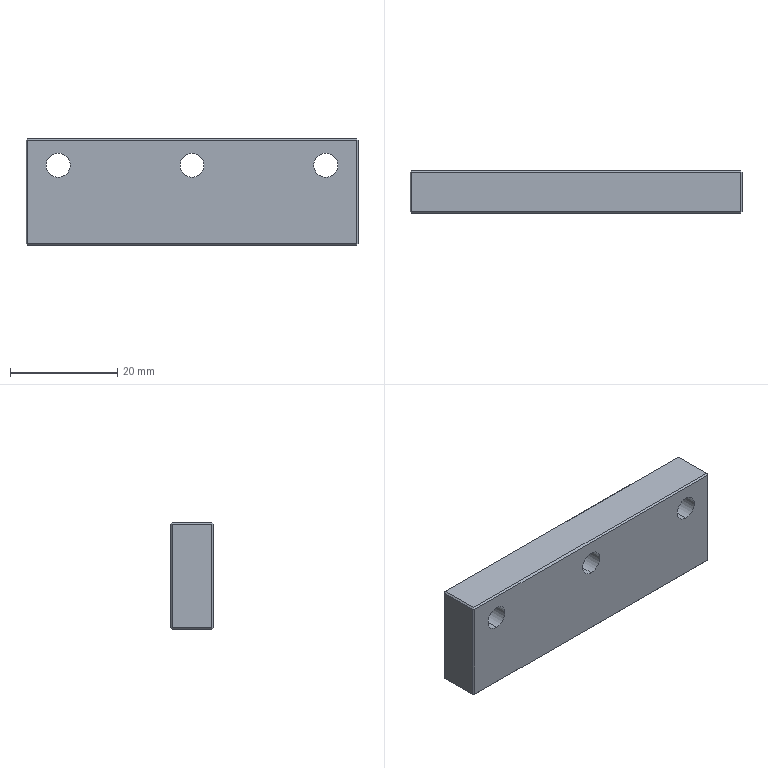Part | SolidWorks | features Chamfer 1, Extrusion 1, HoleWzd 1 | 1 solid | 41 faces | box 62 x 8 x 20 mm | volume 9069 mm3 | plane 29 | cylinder 12 | commonest cylinder face diameters 4.5 x6 8 x6
STEP:
#1=CARTESIAN_POINT('',(-25.,3.6,1.));
#2=VERTEX_POINT('',#1);
#3=CARTESIAN_POINT('',(-25.,3.6,9.));
#4=VERTEX_POINT('',#3);
#5=CARTESIAN_POINT('',(-25.,3.6,5.));
#6=DIRECTION('',(0.,1.,0.));
#7=DIRECTION('',(0.,0.,1.));
#8=AXIS2_PLACEMENT_3D('',#5,#6,#7);
#9=CIRCLE('',#8,4.);
#10=EDGE_CURVE('',#2,#4,#9,.T.);
#11=ORIENTED_EDGE('',*,*,#10,.F.);
#12=CARTESIAN_POINT('',(-25.,8.,1.));
#13=VERTEX_POINT('',#12);
#14=CARTESIAN_POINT('',(-25.,8.,1.));
#15=DIRECTION('',(0.,1.,0.));
#16=VECTOR('',#15,1000.);
#17=LINE('',#14,#16);
#18=EDGE_CURVE('',#2,#13,#17,.T.);
#19=ORIENTED_EDGE('',*,*,#18,.T.);
#20=CARTESIAN_POINT('',(-25.,8.,9.));
#21=VERTEX_POINT('',#20);
#22=CARTESIAN_POINT('',(-25.,8.,5.));
#23=DIRECTION('',(0.,1.,0.));
#24=DIRECTION('',(0.,0.,1.));
#25=AXIS2_PLACEMENT_3D('',#22,#23,#24);
#26=CIRCLE('',#25,4.);
#27=EDGE_CURVE('',#13,#21,#26,.T.);
#28=ORIENTED_EDGE('',*,*,#27,.T.);
#29=CARTESIAN_POINT('',(-25.,8.,9.));
#30=DIRECTION('',(0.,1.,0.));
#31=VECTOR('',#30,1000.);
#32=LINE('',#29,#31);
#33=EDGE_CURVE('',#4,#21,#32,.T.);
#34=ORIENTED_EDGE('',*,*,#33,.F.);
#35=EDGE_LOOP('',(#11,#19,#28,#34));
#36=FACE_OUTER_BOUND('',#35,.T.);
#37=CARTESIAN_POINT('',(-25.,8.,5.));
#38=DIRECTION('',(0.,1.,0.));
#39=DIRECTION('',(0.,0.,1.));
#40=AXIS2_PLACEMENT_3D('',#37,#38,#39);
#41=CYLINDRICAL_SURFACE('',#40,4.);
#42=ADVANCED_FACE('',(#36),#41,.F.);
#43=CARTESIAN_POINT('',(-25.,0.,2.75));
#44=VERTEX_POINT('',#43);
#45=CARTESIAN_POINT('',(-25.,0.,7.25));
#46=VERTEX_POINT('',#45);
#47=CARTESIAN_POINT('',(-25.,0.,5.));
#48=DIRECTION('',(0.,1.,0.));
#49=DIRECTION('',(0.,0.,1.));
#50=AXIS2_PLACEMENT_3D('',#47,#48,#49);
#51=CIRCLE('',#50,2.25);
#52=EDGE_CURVE('',#44,#46,#51,.T.);
#53=ORIENTED_EDGE('',*,*,#52,.F.);
#54=CARTESIAN_POINT('',(-25.,3.6,2.75));
#55=VERTEX_POINT('',#54);
#56=CARTESIAN_POINT('',(-25.,8.,2.75));
#57=DIRECTION('',(0.,1.,0.));
#58=VECTOR('',#57,1000.);
#59=LINE('',#56,#58);
#60=EDGE_CURVE('',#44,#55,#59,.T.);
#61=ORIENTED_EDGE('',*,*,#60,.T.);
#62=CARTESIAN_POINT('',(-25.,3.6,7.25));
#63=VERTEX_POINT('',#62);
#64=CARTESIAN_POINT('',(-25.,3.6,5.));
#65=DIRECTION('',(0.,1.,0.));
#66=DIRECTION('',(0.,0.,1.));
#67=AXIS2_PLACEMENT_3D('',#64,#65,#66);
#68=CIRCLE('',#67,2.25);
#69=EDGE_CURVE('',#55,#63,#68,.T.);
#70=ORIENTED_EDGE('',*,*,#69,.T.);
#71=CARTESIAN_POINT('',(-25.,8.,7.25));
#72=DIRECTION('',(0.,1.,0.));
#73=VECTOR('',#72,1000.);
#74=LINE('',#71,#73);
#75=EDGE_CURVE('',#46,#63,#74,.T.);
#76=ORIENTED_EDGE('',*,*,#75,.F.);
#77=EDGE_LOOP('',(#53,#61,#70,#76));
#78=FACE_OUTER_BOUND('',#77,.T.);
#79=CARTESIAN_POINT('',(-25.,8.,5.));
#80=DIRECTION('',(0.,1.,0.));
#81=DIRECTION('',(0.,0.,1.));
#82=AXIS2_PLACEMENT_3D('',#79,#80,#81);
#83=CYLINDRICAL_SURFACE('',#82,2.25);
#84=ADVANCED_FACE('',(#78),#83,.F.);
#85=CARTESIAN_POINT('',(0.,3.6,1.));
#86=VERTEX_POINT('',#85);
#87=CARTESIAN_POINT('',(0.,3.6,9.));
#88=VERTEX_POINT('',#87);
#89=CARTESIAN_POINT('',(0.,3.6,5.));
#90=DIRECTION('',(0.,1.,0.));
#91=DIRECTION('',(0.,0.,1.));
#92=AXIS2_PLACEMENT_3D('',#89,#90,#91);
#93=CIRCLE('',#92,4.);
#94=EDGE_CURVE('',#86,#88,#93,.T.);
#95=ORIENTED_EDGE('',*,*,#94,.F.);
#96=CARTESIAN_POINT('',(0.,8.,1.));
#97=VERTEX_POINT('',#96);
#98=CARTESIAN_POINT('',(0.,8.,1.));
#99=DIRECTION('',(0.,1.,0.));
#100=VECTOR('',#99,1000.);
#101=LINE('',#98,#100);
#102=EDGE_CURVE('',#86,#97,#101,.T.);
#103=ORIENTED_EDGE('',*,*,#102,.T.);
#104=CARTESIAN_POINT('',(0.,8.,9.));
#105=VERTEX_POINT('',#104);
#106=CARTESIAN_POINT('',(0.,8.,5.));
#107=DIRECTION('',(0.,1.,0.));
#108=DIRECTION('',(0.,0.,1.));
#109=AXIS2_PLACEMENT_3D('',#106,#107,#108);
#110=CIRCLE('',#109,4.);
#111=EDGE_CURVE('',#97,#105,#110,.T.);
#112=ORIENTED_EDGE('',*,*,#111,.T.);
#113=CARTESIAN_POINT('',(0.,8.,9.));
#114=DIRECTION('',(0.,1.,0.));
#115=VECTOR('',#114,1000.);
#116=LINE('',#113,#115);
#117=EDGE_CURVE('',#88,#105,#116,.T.);
#118=ORIENTED_EDGE('',*,*,#117,.F.);
#119=EDGE_LOOP('',(#95,#103,#112,#118));
#120=FACE_OUTER_BOUND('',#119,.T.);
#121=CARTESIAN_POINT('',(0.,8.,5.));
#122=DIRECTION('',(0.,1.,0.));
#123=DIRECTION('',(0.,0.,1.));
#124=AXIS2_PLACEMENT_3D('',#121,#122,#123);
#125=CYLINDRICAL_SURFACE('',#124,4.);
#126=ADVANCED_FACE('',(#120),#125,.F.);
#127=CARTESIAN_POINT('',(0.,0.,2.75));
#128=VERTEX_POINT('',#127);
#129=CARTESIAN_POINT('',(0.,0.,7.25));
#130=VERTEX_POINT('',#129);
#131=CARTESIAN_POINT('',(0.,0.,5.));
#132=DIRECTION('',(0.,1.,0.));
#133=DIRECTION('',(0.,0.,1.));
#134=AXIS2_PLACEMENT_3D('',#131,#132,#133);
#135=CIRCLE('',#134,2.25);
#136=EDGE_CURVE('',#128,#130,#135,.T.);
#137=ORIENTED_EDGE('',*,*,#136,.F.);
#138=CARTESIAN_POINT('',(0.,3.6,2.75));
#139=VERTEX_POINT('',#138);
#140=CARTESIAN_POINT('',(0.,8.,2.75));
#141=DIRECTION('',(0.,1.,0.));
#142=VECTOR('',#141,1000.);
#143=LINE('',#140,#142);
#144=EDGE_CURVE('',#128,#139,#143,.T.);
#145=ORIENTED_EDGE('',*,*,#144,.T.);
#146=CARTESIAN_POINT('',(0.,3.6,7.25));
#147=VERTEX_POINT('',#146);
#148=CARTESIAN_POINT('',(0.,3.6,5.));
#149=DIRECTION('',(0.,1.,0.));
#150=DIRECTION('',(0.,0.,1.));
#151=AXIS2_PLACEMENT_3D('',#148,#149,#150);
#152=CIRCLE('',#151,2.25);
#153=EDGE_CURVE('',#139,#147,#152,.T.);
#154=ORIENTED_EDGE('',*,*,#153,.T.);
#155=CARTESIAN_POINT('',(0.,8.,7.25));
#156=DIRECTION('',(0.,1.,0.));
#157=VECTOR('',#156,1000.);
#158=LINE('',#155,#157);
#159=EDGE_CURVE('',#130,#147,#158,.T.);
#160=ORIENTED_EDGE('',*,*,#159,.F.);
#161=EDGE_LOOP('',(#137,#145,#154,#160));
#162=FACE_OUTER_BOUND('',#161,.T.);
#163=CARTESIAN_POINT('',(0.,8.,5.));
#164=DIRECTION('',(0.,1.,0.));
#165=DIRECTION('',(0.,0.,1.));
#166=AXIS2_PLACEMENT_3D('',#163,#164,#165);
#167=CYLINDRICAL_SURFACE('',#166,2.25);
#168=ADVANCED_FACE('',(#162),#167,.F.);
#169=CARTESIAN_POINT('',(25.,3.6,1.));
#170=VERTEX_POINT('',#169);
#171=CARTESIAN_POINT('',(25.,3.6,9.));
#172=VERTEX_POINT('',#171);
#173=CARTESIAN_POINT('',(25.,3.6,5.));
#174=DIRECTION('',(0.,1.,0.));
#175=DIRECTION('',(0.,0.,1.));
#176=AXIS2_PLACEMENT_3D('',#173,#174,#175);
#177=CIRCLE('',#176,4.);
#178=EDGE_CURVE('',#170,#172,#177,.T.);
#179=ORIENTED_EDGE('',*,*,#178,.F.);
#180=CARTESIAN_POINT('',(25.,8.,1.));
#181=VERTEX_POINT('',#180);
#182=CARTESIAN_POINT('',(25.,8.,1.));
#183=DIRECTION('',(0.,1.,0.));
#184=VECTOR('',#183,1000.);
#185=LINE('',#182,#184);
#186=EDGE_CURVE('',#170,#181,#185,.T.);
#187=ORIENTED_EDGE('',*,*,#186,.T.);
#188=CARTESIAN_POINT('',(25.,8.,9.));
#189=VERTEX_POINT('',#188);
#190=CARTESIAN_POINT('',(25.,8.,5.));
#191=DIRECTION('',(0.,1.,0.));
#192=DIRECTION('',(0.,0.,1.));
#193=AXIS2_PLACEMENT_3D('',#190,#191,#192);
#194=CIRCLE('',#193,4.);
#195=EDGE_CURVE('',#181,#189,#194,.T.);
#196=ORIENTED_EDGE('',*,*,#195,.T.);
#197=CARTESIAN_POINT('',(25.,8.,9.));
#198=DIRECTION('',(0.,1.,0.));
#199=VECTOR('',#198,1000.);
#200=LINE('',#197,#199);
#201=EDGE_CURVE('',#172,#189,#200,.T.);
#202=ORIENTED_EDGE('',*,*,#201,.F.);
#203=EDGE_LOOP('',(#179,#187,#196,#202));
#204=FACE_OUTER_BOUND('',#203,.T.);
#205=CARTESIAN_POINT('',(25.,8.,5.));
#206=DIRECTION('',(0.,1.,0.));
#207=DIRECTION('',(0.,0.,1.));
#208=AXIS2_PLACEMENT_3D('',#205,#206,#207);
#209=CYLINDRICAL_SURFACE('',#208,4.);
#210=ADVANCED_FACE('',(#204),#209,.F.);
#211=CARTESIAN_POINT('',(25.,0.,2.75));
#212=VERTEX_POINT('',#211);
#213=CARTESIAN_POINT('',(25.,0.,7.25));
#214=VERTEX_POINT('',#213);
#215=CARTESIAN_POINT('',(25.,0.,5.));
#216=DIRECTION('',(0.,1.,0.));
#217=DIRECTION('',(0.,0.,1.));
#218=AXIS2_PLACEMENT_3D('',#215,#216,#217);
#219=CIRCLE('',#218,2.25);
#220=EDGE_CURVE('',#212,#214,#219,.T.);
#221=ORIENTED_EDGE('',*,*,#220,.F.);
#222=CARTESIAN_POINT('',(25.,3.6,2.75));
#223=VERTEX_POINT('',#222);
#224=CARTESIAN_POINT('',(25.,8.,2.75));
#225=DIRECTION('',(0.,1.,0.));
#226=VECTOR('',#225,1000.);
#227=LINE('',#224,#226);
#228=EDGE_CURVE('',#212,#223,#227,.T.);
#229=ORIENTED_EDGE('',*,*,#228,.T.);
#230=CARTESIAN_POINT('',(25.,3.6,7.25));
#231=VERTEX_POINT('',#230);
#232=CARTESIAN_POINT('',(25.,3.6,5.));
#233=DIRECTION('',(0.,1.,0.));
#234=DIRECTION('',(0.,0.,1.));
#235=AXIS2_PLACEMENT_3D('',#232,#233,#234);
#236=CIRCLE('',#235,2.25);
#237=EDGE_CURVE('',#223,#231,#236,.T.);
#238=ORIENTED_EDGE('',*,*,#237,.T.);
#239=CARTESIAN_POINT('',(25.,8.,7.25));
#240=DIRECTION('',(0.,1.,0.));
#241=VECTOR('',#240,1000.);
#242=LINE('',#239,#241);
#243=EDGE_CURVE('',#214,#231,#242,.T.);
#244=ORIENTED_EDGE('',*,*,#243,.F.);
#245=EDGE_LOOP('',(#221,#229,#238,#244));
#246=FACE_OUTER_BOUND('',#245,.T.);
#247=CARTESIAN_POINT('',(25.,8.,5.));
#248=DIRECTION('',(0.,1.,0.));
#249=DIRECTION('',(0.,0.,1.));
#250=AXIS2_PLACEMENT_3D('',#247,#248,#249);
#251=CYLINDRICAL_SURFACE('',#250,2.25);
#252=ADVANCED_FACE('',(#246),#251,.F.);
#253=CARTESIAN_POINT('',(31.,0.3,-9.7));
#254=VERTEX_POINT('',#253);
#255=CARTESIAN_POINT('',(31.,7.7,-9.7));
#256=VERTEX_POINT('',#255);
#257=CARTESIAN_POINT('',(31.,8.,-9.7));
#258=DIRECTION('',(0.,1.,0.));
#259=VECTOR('',#258,1000.);
#260=LINE('',#257,#259);
#261=EDGE_CURVE('',#254,#256,#260,.T.);
#262=ORIENTED_EDGE('',*,*,#261,.T.);
#263=CARTESIAN_POINT('',(31.,7.7,9.7));
#264=VERTEX_POINT('',#263);
#265=CARTESIAN_POINT('',(31.,7.7,10.));
#266=DIRECTION('',(0.,0.,1.));
#267=VECTOR('',#266,1000.);
#268=LINE('',#265,#267);
#269=EDGE_CURVE('',#256,#264,#268,.T.);
#270=ORIENTED_EDGE('',*,*,#269,.T.);
#271=CARTESIAN_POINT('',(31.,0.3,9.7));
#272=VERTEX_POINT('',#271);
#273=CARTESIAN_POINT('',(31.,8.,9.7));
#274=DIRECTION('',(0.,-1.,0.));
#275=VECTOR('',#274,1000.);
#276=LINE('',#273,#275);
#277=EDGE_CURVE('',#264,#272,#276,.T.);
#278=ORIENTED_EDGE('',*,*,#277,.T.);
#279=CARTESIAN_POINT('',(31.,0.3,-10.));
#280=DIRECTION('',(0.,0.,-1.));
#281=VECTOR('',#280,1000.);
#282=LINE('',#279,#281);
#283=EDGE_CURVE('',#272,#254,#282,.T.);
#284=ORIENTED_EDGE('',*,*,#283,.T.);
#285=EDGE_LOOP('',(#262,#270,#278,#284));
#286=FACE_OUTER_BOUND('',#285,.T.);
#287=CARTESIAN_POINT('',(31.,8.,-10.));
#288=DIRECTION('',(-1.,0.,0.));
#289=DIRECTION('',(0.,0.,1.));
#290=AXIS2_PLACEMENT_3D('',#287,#288,#289);
#291=PLANE('',#290);
#292=ADVANCED_FACE('',(#286),#291,.F.);
#293=CARTESIAN_POINT('',(-30.7,0.3,-10.));
#294=VERTEX_POINT('',#293);
#295=CARTESIAN_POINT('',(-30.7,7.7,-10.));
#296=VERTEX_POINT('',#295);
#297=CARTESIAN_POINT('',(-30.7,8.,-10.));
#298=DIRECTION('',(0.,1.,0.));
#299=VECTOR('',#298,1000.);
#300=LINE('',#297,#299);
#301=EDGE_CURVE('',#294,#296,#300,.T.);
#302=ORIENTED_EDGE('',*,*,#301,.T.);
#303=CARTESIAN_POINT('',(30.7,7.7,-10.));
#304=VERTEX_POINT('',#303);
#305=CARTESIAN_POINT('',(31.,7.7,-10.));
#306=DIRECTION('',(1.,0.,0.));
#307=VECTOR('',#306,1000.);
#308=LINE('',#305,#307);
#309=EDGE_CURVE('',#296,#304,#308,.T.);
#310=ORIENTED_EDGE('',*,*,#309,.T.);
#311=CARTESIAN_POINT('',(30.7,0.3,-10.));
#312=VERTEX_POINT('',#311);
#313=CARTESIAN_POINT('',(30.7,8.,-10.));
#314=DIRECTION('',(0.,-1.,0.));
#315=VECTOR('',#314,1000.);
#316=LINE('',#313,#315);
#317=EDGE_CURVE('',#304,#312,#316,.T.);
#318=ORIENTED_EDGE('',*,*,#317,.T.);
#319=CARTESIAN_POINT('',(-31.,0.3,-10.));
#320=DIRECTION('',(-1.,0.,0.));
#321=VECTOR('',#320,1000.);
#322=LINE('',#319,#321);
#323=EDGE_CURVE('',#312,#294,#322,.T.);
#324=ORIENTED_EDGE('',*,*,#323,.T.);
#325=EDGE_LOOP('',(#302,#310,#318,#324));
#326=FACE_OUTER_BOUND('',#325,.T.);
#327=CARTESIAN_POINT('',(-31.,8.,-10.));
#328=DIRECTION('',(0.,0.,1.));
#329=DIRECTION('',(1.,0.,0.));
#330=AXIS2_PLACEMENT_3D('',#327,#328,#329);
#331=PLANE('',#330);
#332=ADVANCED_FACE('',(#326),#331,.F.);
#333=CARTESIAN_POINT('',(-31.,7.7,9.7));
#334=VERTEX_POINT('',#333);
#335=CARTESIAN_POINT('',(-31.,7.7,-9.7));
#336=VERTEX_POINT('',#335);
#337=CARTESIAN_POINT('',(-31.,7.7,-10.));
#338=DIRECTION('',(0.,0.,-1.));
#339=VECTOR('',#338,1000.);
#340=LINE('',#337,#339);
#341=EDGE_CURVE('',#334,#336,#340,.T.);
#342=ORIENTED_EDGE('',*,*,#341,.T.);
#343=CARTESIAN_POINT('',(-31.,0.3,-9.7));
#344=VERTEX_POINT('',#343);
#345=CARTESIAN_POINT('',(-31.,8.,-9.7));
#346=DIRECTION('',(0.,-1.,0.));
#347=VECTOR('',#346,1000.);
#348=LINE('',#345,#347);
#349=EDGE_CURVE('',#336,#344,#348,.T.);
#350=ORIENTED_EDGE('',*,*,#349,.T.);
#351=CARTESIAN_POINT('',(-31.,0.3,9.7));
#352=VERTEX_POINT('',#351);
#353=CARTESIAN_POINT('',(-31.,0.3,-10.));
#354=DIRECTION('',(0.,0.,1.));
#355=VECTOR('',#354,1000.);
#356=LINE('',#353,#355);
#357=EDGE_CURVE('',#344,#352,#356,.T.);
#358=ORIENTED_EDGE('',*,*,#357,.T.);
#359=CARTESIAN_POINT('',(-31.,8.,9.7));
#360=DIRECTION('',(0.,1.,0.));
#361=VECTOR('',#360,1000.);
#362=LINE('',#359,#361);
#363=EDGE_CURVE('',#352,#334,#362,.T.);
#364=ORIENTED_EDGE('',*,*,#363,.T.);
#365=EDGE_LOOP('',(#342,#350,#358,#364));
#366=FACE_OUTER_BOUND('',#365,.T.);
#367=CARTESIAN_POINT('',(-31.,8.,-10.));
#368=DIRECTION('',(1.,0.,0.));
#369=DIRECTION('',(0.,0.,-1.));
#370=AXIS2_PLACEMENT_3D('',#367,#368,#369);
#371=PLANE('',#370);
#372=ADVANCED_FACE('',(#366),#371,.F.);
#373=CARTESIAN_POINT('',(30.7,7.7,10.));
#374=VERTEX_POINT('',#373);
#375=CARTESIAN_POINT('',(-30.7,7.7,10.));
#376=VERTEX_POINT('',#375);
#377=CARTESIAN_POINT('',(-31.,7.7,10.));
#378=DIRECTION('',(-1.,0.,0.));
#379=VECTOR('',#378,1000.);
#380=LINE('',#377,#379);
#381=EDGE_CURVE('',#374,#376,#380,.T.);
#382=ORIENTED_EDGE('',*,*,#381,.T.);
#383=CARTESIAN_POINT('',(-30.7,0.3,10.));
#384=VERTEX_POINT('',#383);
#385=CARTESIAN_POINT('',(-30.7,8.,10.));
#386=DIRECTION('',(0.,-1.,0.));
#387=VECTOR('',#386,1000.);
#388=LINE('',#385,#387);
#389=EDGE_CURVE('',#376,#384,#388,.T.);
#390=ORIENTED_EDGE('',*,*,#389,.T.);
#391=CARTESIAN_POINT('',(30.7,0.3,10.));
#392=VERTEX_POINT('',#391);
#393=CARTESIAN_POINT('',(-31.,0.3,10.));
#394=DIRECTION('',(1.,0.,0.));
#395=VECTOR('',#394,1000.);
#396=LINE('',#393,#395);
#397=EDGE_CURVE('',#384,#392,#396,.T.);
#398=ORIENTED_EDGE('',*,*,#397,.T.);
#399=CARTESIAN_POINT('',(30.7,8.,10.));
#400=DIRECTION('',(0.,1.,0.));
#401=VECTOR('',#400,1000.);
#402=LINE('',#399,#401);
#403=EDGE_CURVE('',#392,#374,#402,.T.);
#404=ORIENTED_EDGE('',*,*,#403,.T.);
#405=EDGE_LOOP('',(#382,#390,#398,#404));
#406=FACE_OUTER_BOUND('',#405,.T.);
#407=CARTESIAN_POINT('',(-31.,8.,10.));
#408=DIRECTION('',(0.,0.,-1.));
#409=DIRECTION('',(-1.,0.,0.));
#410=AXIS2_PLACEMENT_3D('',#407,#408,#409);
#411=PLANE('',#410);
#412=ADVANCED_FACE('',(#406),#411,.F.);
#413=CARTESIAN_POINT('',(30.7,8.,-9.7));
#414=VERTEX_POINT('',#413);
#415=CARTESIAN_POINT('',(-30.7,8.,-9.7));
#416=VERTEX_POINT('',#415);
#417=CARTESIAN_POINT('',(-31.,8.,-9.7));
#418=DIRECTION('',(-1.,0.,0.));
#419=VECTOR('',#418,1000.);
#420=LINE('',#417,#419);
#421=EDGE_CURVE('',#414,#416,#420,.T.);
#422=ORIENTED_EDGE('',*,*,#421,.T.);
#423=CARTESIAN_POINT('',(-30.7,8.,9.7));
#424=VERTEX_POINT('',#423);
#425=CARTESIAN_POINT('',(-30.7,8.,10.));
#426=DIRECTION('',(0.,0.,1.));
#427=VECTOR('',#426,1000.);
#428=LINE('',#425,#427);
#429=EDGE_CURVE('',#416,#424,#428,.T.);
#430=ORIENTED_EDGE('',*,*,#429,.T.);
#431=CARTESIAN_POINT('',(30.7,8.,9.7));
#432=VERTEX_POINT('',#431);
#433=CARTESIAN_POINT('',(31.,8.,9.7));
#434=DIRECTION('',(1.,0.,0.));
#435=VECTOR('',#434,1000.);
#436=LINE('',#433,#435);
#437=EDGE_CURVE('',#424,#432,#436,.T.);
#438=ORIENTED_EDGE('',*,*,#437,.T.);
#439=CARTESIAN_POINT('',(30.7,8.,-10.));
#440=DIRECTION('',(0.,0.,-1.));
#441=VECTOR('',#440,1000.);
#442=LINE('',#439,#441);
#443=EDGE_CURVE('',#432,#414,#442,.T.);
#444=ORIENTED_EDGE('',*,*,#443,.T.);
#445=EDGE_LOOP('',(#422,#430,#438,#444));
#446=FACE_OUTER_BOUND('',#445,.T.);
#447=CARTESIAN_POINT('',(-25.,8.,5.));
#448=DIRECTION('',(0.,1.,0.));
#449=DIRECTION('',(0.,0.,1.));
#450=AXIS2_PLACEMENT_3D('',#447,#448,#449);
#451=CIRCLE('',#450,4.);
#452=EDGE_CURVE('',#21,#13,#451,.T.);
#453=ORIENTED_EDGE('',*,*,#452,.F.);
#454=ORIENTED_EDGE('',*,*,#27,.F.);
#455=EDGE_LOOP('',(#453,#454));
#456=FACE_BOUND('',#455,.T.);
#457=CARTESIAN_POINT('',(0.,8.,5.));
#458=DIRECTION('',(0.,1.,0.));
#459=DIRECTION('',(0.,0.,1.));
#460=AXIS2_PLACEMENT_3D('',#457,#458,#459);
#461=CIRCLE('',#460,4.);
#462=EDGE_CURVE('',#105,#97,#461,.T.);
#463=ORIENTED_EDGE('',*,*,#462,.F.);
#464=ORIENTED_EDGE('',*,*,#111,.F.);
#465=EDGE_LOOP('',(#463,#464));
#466=FACE_BOUND('',#465,.T.);
#467=CARTESIAN_POINT('',(25.,8.,5.));
#468=DIRECTION('',(0.,1.,0.));
#469=DIRECTION('',(0.,0.,1.));
#470=AXIS2_PLACEMENT_3D('',#467,#468,#469);
#471=CIRCLE('',#470,4.);
#472=EDGE_CURVE('',#189,#181,#471,.T.);
#473=ORIENTED_EDGE('',*,*,#472,.F.);
#474=ORIENTED_EDGE('',*,*,#195,.F.);
#475=EDGE_LOOP('',(#473,#474));
#476=FACE_BOUND('',#475,.T.);
#477=CARTESIAN_POINT('',(0.,8.,0.));
#478=DIRECTION('',(0.,1.,0.));
#479=DIRECTION('',(0.,0.,1.));
#480=AXIS2_PLACEMENT_3D('',#477,#478,#479);
#481=PLANE('',#480);
#482=ADVANCED_FACE('',(#446,#456,#466,#476),#481,.T.);
#483=CARTESIAN_POINT('',(30.7,0.,9.7));
#484=VERTEX_POINT('',#483);
#485=CARTESIAN_POINT('',(-30.7,0.,9.7));
#486=VERTEX_POINT('',#485);
#487=CARTESIAN_POINT('',(0.,0.,9.7));
#488=DIRECTION('',(-1.,0.,0.));
#489=VECTOR('',#488,1000.);
#490=LINE('',#487,#489);
#491=EDGE_CURVE('',#484,#486,#490,.T.);
#492=ORIENTED_EDGE('',*,*,#491,.T.);
#493=CARTESIAN_POINT('',(-30.7,0.,-9.7));
#494=VERTEX_POINT('',#493);
#495=CARTESIAN_POINT('',(-30.7,0.,0.));
#496=DIRECTION('',(0.,0.,-1.));
#497=VECTOR('',#496,1000.);
#498=LINE('',#495,#497);
#499=EDGE_CURVE('',#486,#494,#498,.T.);
#500=ORIENTED_EDGE('',*,*,#499,.T.);
#501=CARTESIAN_POINT('',(30.7,0.,-9.7));
#502=VERTEX_POINT('',#501);
#503=CARTESIAN_POINT('',(0.,0.,-9.7));
#504=DIRECTION('',(1.,0.,0.));
#505=VECTOR('',#504,1000.);
#506=LINE('',#503,#505);
#507=EDGE_CURVE('',#494,#502,#506,.T.);
#508=ORIENTED_EDGE('',*,*,#507,.T.);
#509=CARTESIAN_POINT('',(30.7,0.,0.));
#510=DIRECTION('',(0.,0.,1.));
#511=VECTOR('',#510,1000.);
#512=LINE('',#509,#511);
#513=EDGE_CURVE('',#502,#484,#512,.T.);
#514=ORIENTED_EDGE('',*,*,#513,.T.);
#515=EDGE_LOOP('',(#492,#500,#508,#514));
#516=FACE_OUTER_BOUND('',#515,.T.);
#517=CARTESIAN_POINT('',(-25.,0.,5.));
#518=DIRECTION('',(0.,1.,0.));
#519=DIRECTION('',(0.,0.,1.));
#520=AXIS2_PLACEMENT_3D('',#517,#518,#519);
#521=CIRCLE('',#520,2.25);
#522=EDGE_CURVE('',#46,#44,#521,.T.);
#523=ORIENTED_EDGE('',*,*,#522,.T.);
#524=ORIENTED_EDGE('',*,*,#52,.T.);
#525=EDGE_LOOP('',(#523,#524));
#526=FACE_BOUND('',#525,.T.);
#527=CARTESIAN_POINT('',(0.,0.,5.));
#528=DIRECTION('',(0.,1.,0.));
#529=DIRECTION('',(0.,0.,1.));
#530=AXIS2_PLACEMENT_3D('',#527,#528,#529);
#531=CIRCLE('',#530,2.25);
#532=EDGE_CURVE('',#130,#128,#531,.T.);
#533=ORIENTED_EDGE('',*,*,#532,.T.);
#534=ORIENTED_EDGE('',*,*,#136,.T.);
#535=EDGE_LOOP('',(#533,#534));
#536=FACE_BOUND('',#535,.T.);
#537=CARTESIAN_POINT('',(25.,0.,5.));
#538=DIRECTION('',(0.,1.,0.));
#539=DIRECTION('',(0.,0.,1.));
#540=AXIS2_PLACEMENT_3D('',#537,#538,#539);
#541=CIRCLE('',#540,2.25);
#542=EDGE_CURVE('',#214,#212,#541,.T.);
#543=ORIENTED_EDGE('',*,*,#542,.T.);
#544=ORIENTED_EDGE('',*,*,#220,.T.);
#545=EDGE_LOOP('',(#543,#544));
#546=FACE_BOUND('',#545,.T.);
#547=CARTESIAN_POINT('',(0.,0.,0.));
#548=DIRECTION('',(0.,1.,0.));
#549=DIRECTION('',(0.,0.,1.));
#550=AXIS2_PLACEMENT_3D('',#547,#548,#549);
#551=PLANE('',#550);
#552=ADVANCED_FACE('',(#516,#526,#536,#546),#551,.F.);
#553=ORIENTED_EDGE('',*,*,#228,.F.);
#554=ORIENTED_EDGE('',*,*,#542,.F.);
#555=ORIENTED_EDGE('',*,*,#243,.T.);
#556=CARTESIAN_POINT('',(25.,3.6,5.));
#557=DIRECTION('',(0.,1.,0.));
#558=DIRECTION('',(0.,0.,1.));
#559=AXIS2_PLACEMENT_3D('',#556,#557,#558);
#560=CIRCLE('',#559,2.25);
#561=EDGE_CURVE('',#231,#223,#560,.T.);
#562=ORIENTED_EDGE('',*,*,#561,.T.);
#563=EDGE_LOOP('',(#553,#554,#555,#562));
#564=FACE_OUTER_BOUND('',#563,.T.);
#565=CARTESIAN_POINT('',(25.,8.,5.));
#566=DIRECTION('',(0.,1.,0.));
#567=DIRECTION('',(0.,0.,1.));
#568=AXIS2_PLACEMENT_3D('',#565,#566,#567);
#569=CYLINDRICAL_SURFACE('',#568,2.25);
#570=ADVANCED_FACE('',(#564),#569,.F.);
#571=ORIENTED_EDGE('',*,*,#561,.F.);
#572=ORIENTED_EDGE('',*,*,#237,.F.);
#573=EDGE_LOOP('',(#571,#572));
#574=FACE_BOUND('',#573,.T.);
#575=CARTESIAN_POINT('',(25.,3.6,5.));
#576=DIRECTION('',(0.,1.,0.));
#577=DIRECTION('',(0.,0.,1.));
#578=AXIS2_PLACEMENT_3D('',#575,#576,#577);
#579=CIRCLE('',#578,4.);
#580=EDGE_CURVE('',#172,#170,#579,.T.);
#581=ORIENTED_EDGE('',*,*,#580,.T.);
#582=ORIENTED_EDGE('',*,*,#178,.T.);
#583=EDGE_LOOP('',(#581,#582));
#584=FACE_OUTER_BOUND('',#583,.T.);
#585=CARTESIAN_POINT('',(27.25,3.6,5.));
#586=DIRECTION('',(0.,-1.,0.));
#587=DIRECTION('',(0.,0.,-1.));
#588=AXIS2_PLACEMENT_3D('',#585,#586,#587);
#589=PLANE('',#588);
#590=ADVANCED_FACE('',(#574,#584),#589,.F.);
#591=ORIENTED_EDGE('',*,*,#186,.F.);
#592=ORIENTED_EDGE('',*,*,#580,.F.);
#593=ORIENTED_EDGE('',*,*,#201,.T.);
#594=ORIENTED_EDGE('',*,*,#472,.T.);
#595=EDGE_LOOP('',(#591,#592,#593,#594));
#596=FACE_OUTER_BOUND('',#595,.T.);
#597=CARTESIAN_POINT('',(25.,8.,5.));
#598=DIRECTION('',(0.,1.,0.));
#599=DIRECTION('',(0.,0.,1.));
#600=AXIS2_PLACEMENT_3D('',#597,#598,#599);
#601=CYLINDRICAL_SURFACE('',#600,4.);
#602=ADVANCED_FACE('',(#596),#601,.F.);
#603=ORIENTED_EDGE('',*,*,#144,.F.);
#604=ORIENTED_EDGE('',*,*,#532,.F.);
#605=ORIENTED_EDGE('',*,*,#159,.T.);
#606=CARTESIAN_POINT('',(0.,3.6,5.));
#607=DIRECTION('',(0.,1.,0.));
#608=DIRECTION('',(0.,0.,1.));
#609=AXIS2_PLACEMENT_3D('',#606,#607,#608);
#610=CIRCLE('',#609,2.25);
#611=EDGE_CURVE('',#147,#139,#610,.T.);
#612=ORIENTED_EDGE('',*,*,#611,.T.);
#613=EDGE_LOOP('',(#603,#604,#605,#612));
#614=FACE_OUTER_BOUND('',#613,.T.);
#615=CARTESIAN_POINT('',(0.,8.,5.));
#616=DIRECTION('',(0.,1.,0.));
#617=DIRECTION('',(0.,0.,1.));
#618=AXIS2_PLACEMENT_3D('',#615,#616,#617);
#619=CYLINDRICAL_SURFACE('',#618,2.25);
#620=ADVANCED_FACE('',(#614),#619,.F.);
#621=ORIENTED_EDGE('',*,*,#611,.F.);
#622=ORIENTED_EDGE('',*,*,#153,.F.);
#623=EDGE_LOOP('',(#621,#622));
#624=FACE_BOUND('',#623,.T.);
#625=CARTESIAN_POINT('',(0.,3.6,5.));
#626=DIRECTION('',(0.,1.,0.));
#627=DIRECTION('',(0.,0.,1.));
#628=AXIS2_PLACEMENT_3D('',#625,#626,#627);
#629=CIRCLE('',#628,4.);
#630=EDGE_CURVE('',#88,#86,#629,.T.);
#631=ORIENTED_EDGE('',*,*,#630,.T.);
#632=ORIENTED_EDGE('',*,*,#94,.T.);
#633=EDGE_LOOP('',(#631,#632));
#634=FACE_OUTER_BOUND('',#633,.T.);
#635=CARTESIAN_POINT('',(2.25,3.6,5.));
#636=DIRECTION('',(0.,-1.,0.));
#637=DIRECTION('',(0.,0.,-1.));
#638=AXIS2_PLACEMENT_3D('',#635,#636,#637);
#639=PLANE('',#638);
#640=ADVANCED_FACE('',(#624,#634),#639,.F.);
#641=ORIENTED_EDGE('',*,*,#102,.F.);
#642=ORIENTED_EDGE('',*,*,#630,.F.);
#643=ORIENTED_EDGE('',*,*,#117,.T.);
#644=ORIENTED_EDGE('',*,*,#462,.T.);
#645=EDGE_LOOP('',(#641,#642,#643,#644));
#646=FACE_OUTER_BOUND('',#645,.T.);
#647=CARTESIAN_POINT('',(0.,8.,5.));
#648=DIRECTION('',(0.,1.,0.));
#649=DIRECTION('',(0.,0.,1.));
#650=AXIS2_PLACEMENT_3D('',#647,#648,#649);
#651=CYLINDRICAL_SURFACE('',#650,4.);
#652=ADVANCED_FACE('',(#646),#651,.F.);
#653=ORIENTED_EDGE('',*,*,#60,.F.);
#654=ORIENTED_EDGE('',*,*,#522,.F.);
#655=ORIENTED_EDGE('',*,*,#75,.T.);
#656=CARTESIAN_POINT('',(-25.,3.6,5.));
#657=DIRECTION('',(0.,1.,0.));
#658=DIRECTION('',(0.,0.,1.));
#659=AXIS2_PLACEMENT_3D('',#656,#657,#658);
#660=CIRCLE('',#659,2.25);
#661=EDGE_CURVE('',#63,#55,#660,.T.);
#662=ORIENTED_EDGE('',*,*,#661,.T.);
#663=EDGE_LOOP('',(#653,#654,#655,#662));
#664=FACE_OUTER_BOUND('',#663,.T.);
#665=CARTESIAN_POINT('',(-25.,8.,5.));
#666=DIRECTION('',(0.,1.,0.));
#667=DIRECTION('',(0.,0.,1.));
#668=AXIS2_PLACEMENT_3D('',#665,#666,#667);
#669=CYLINDRICAL_SURFACE('',#668,2.25);
#670=ADVANCED_FACE('',(#664),#669,.F.);
#671=ORIENTED_EDGE('',*,*,#661,.F.);
#672=ORIENTED_EDGE('',*,*,#69,.F.);
#673=EDGE_LOOP('',(#671,#672));
#674=FACE_BOUND('',#673,.T.);
#675=CARTESIAN_POINT('',(-25.,3.6,5.));
#676=DIRECTION('',(0.,1.,0.));
#677=DIRECTION('',(0.,0.,1.));
#678=AXIS2_PLACEMENT_3D('',#675,#676,#677);
#679=CIRCLE('',#678,4.);
#680=EDGE_CURVE('',#4,#2,#679,.T.);
#681=ORIENTED_EDGE('',*,*,#680,.T.);
#682=ORIENTED_EDGE('',*,*,#10,.T.);
#683=EDGE_LOOP('',(#681,#682));
#684=FACE_OUTER_BOUND('',#683,.T.);
#685=CARTESIAN_POINT('',(-22.75,3.6,5.));
#686=DIRECTION('',(0.,-1.,0.));
#687=DIRECTION('',(0.,0.,-1.));
#688=AXIS2_PLACEMENT_3D('',#685,#686,#687);
#689=PLANE('',#688);
#690=ADVANCED_FACE('',(#674,#684),#689,.F.);
#691=ORIENTED_EDGE('',*,*,#18,.F.);
#692=ORIENTED_EDGE('',*,*,#680,.F.);
#693=ORIENTED_EDGE('',*,*,#33,.T.);
#694=ORIENTED_EDGE('',*,*,#452,.T.);
#695=EDGE_LOOP('',(#691,#692,#693,#694));
#696=FACE_OUTER_BOUND('',#695,.T.);
#697=CARTESIAN_POINT('',(-25.,8.,5.));
#698=DIRECTION('',(0.,1.,0.));
#699=DIRECTION('',(0.,0.,1.));
#700=AXIS2_PLACEMENT_3D('',#697,#698,#699);
#701=CYLINDRICAL_SURFACE('',#700,4.);
#702=ADVANCED_FACE('',(#696),#701,.F.);
#703=CARTESIAN_POINT('',(30.7,0.,-9.7));
#704=DIRECTION('',(-0.7071,-0.7071,0.));
#705=VECTOR('',#704,1000.);
#706=LINE('',#703,#705);
#707=EDGE_CURVE('',#254,#502,#706,.T.);
#708=ORIENTED_EDGE('',*,*,#707,.F.);
#709=ORIENTED_EDGE('',*,*,#283,.F.);
#710=CARTESIAN_POINT('',(30.7,0.,9.7));
#711=DIRECTION('',(0.7071,0.7071,0.));
#712=VECTOR('',#711,1000.);
#713=LINE('',#710,#712);
#714=EDGE_CURVE('',#484,#272,#713,.T.);
#715=ORIENTED_EDGE('',*,*,#714,.F.);
#716=ORIENTED_EDGE('',*,*,#513,.F.);
#717=EDGE_LOOP('',(#708,#709,#715,#716));
#718=FACE_OUTER_BOUND('',#717,.T.);
#719=CARTESIAN_POINT('',(31.,0.3,-10.));
#720=DIRECTION('',(-0.7071,0.7071,0.));
#721=DIRECTION('',(0.,0.,-1.));
#722=AXIS2_PLACEMENT_3D('',#719,#720,#721);
#723=PLANE('',#722);
#724=ADVANCED_FACE('',(#718),#723,.F.);
#725=CARTESIAN_POINT('',(30.85,0.3,-9.85));
#726=DIRECTION('',(-0.7071,0.,-0.7071));
#727=VECTOR('',#726,1000.);
#728=LINE('',#725,#727);
#729=EDGE_CURVE('',#254,#312,#728,.T.);
#730=ORIENTED_EDGE('',*,*,#729,.F.);
#731=ORIENTED_EDGE('',*,*,#707,.T.);
#732=CARTESIAN_POINT('',(30.7,0.,-9.7));
#733=DIRECTION('',(0.,-0.7071,0.7071));
#734=VECTOR('',#733,1000.);
#735=LINE('',#732,#734);
#736=EDGE_CURVE('',#312,#502,#735,.T.);
#737=ORIENTED_EDGE('',*,*,#736,.F.);
#738=EDGE_LOOP('',(#730,#731,#737));
#739=FACE_OUTER_BOUND('',#738,.T.);
#740=CARTESIAN_POINT('',(30.7,0.,-9.7));
#741=DIRECTION('',(0.5774,-0.5774,-0.5774));
#742=DIRECTION('',(0.7071,0.7071,0.));
#743=AXIS2_PLACEMENT_3D('',#740,#741,#742);
#744=PLANE('',#743);
#745=ADVANCED_FACE('',(#739),#744,.T.);
#746=CARTESIAN_POINT('',(30.7,0.,9.7));
#747=DIRECTION('',(0.,0.7071,0.7071));
#748=VECTOR('',#747,1000.);
#749=LINE('',#746,#748);
#750=EDGE_CURVE('',#484,#392,#749,.T.);
#751=ORIENTED_EDGE('',*,*,#750,.F.);
#752=ORIENTED_EDGE('',*,*,#714,.T.);
#753=CARTESIAN_POINT('',(30.85,0.3,9.85));
#754=DIRECTION('',(0.7071,0.,-0.7071));
#755=VECTOR('',#754,1000.);
#756=LINE('',#753,#755);
#757=EDGE_CURVE('',#392,#272,#756,.T.);
#758=ORIENTED_EDGE('',*,*,#757,.F.);
#759=EDGE_LOOP('',(#751,#752,#758));
#760=FACE_OUTER_BOUND('',#759,.T.);
#761=CARTESIAN_POINT('',(30.7,0.,9.7));
#762=DIRECTION('',(0.5774,-0.5774,0.5774));
#763=DIRECTION('',(0.7071,0.7071,0.));
#764=AXIS2_PLACEMENT_3D('',#761,#762,#763);
#765=PLANE('',#764);
#766=ADVANCED_FACE('',(#760),#765,.T.);
#767=ORIENTED_EDGE('',*,*,#736,.T.);
#768=ORIENTED_EDGE('',*,*,#507,.F.);
#769=CARTESIAN_POINT('',(-30.7,0.,-9.7));
#770=DIRECTION('',(0.,-0.7071,0.7071));
#771=VECTOR('',#770,1000.);
#772=LINE('',#769,#771);
#773=EDGE_CURVE('',#294,#494,#772,.T.);
#774=ORIENTED_EDGE('',*,*,#773,.F.);
#775=ORIENTED_EDGE('',*,*,#323,.F.);
#776=EDGE_LOOP('',(#767,#768,#774,#775));
#777=FACE_OUTER_BOUND('',#776,.T.);
#778=CARTESIAN_POINT('',(-31.,0.3,-10.));
#779=DIRECTION('',(0.,0.7071,0.7071));
#780=DIRECTION('',(-1.,0.,0.));
#781=AXIS2_PLACEMENT_3D('',#778,#779,#780);
#782=PLANE('',#781);
#783=ADVANCED_FACE('',(#777),#782,.F.);
#784=ORIENTED_EDGE('',*,*,#729,.T.);
#785=ORIENTED_EDGE('',*,*,#317,.F.);
#786=CARTESIAN_POINT('',(30.7,7.7,-10.));
#787=DIRECTION('',(-0.7071,0.,-0.7071));
#788=VECTOR('',#787,1000.);
#789=LINE('',#786,#788);
#790=EDGE_CURVE('',#256,#304,#789,.T.);
#791=ORIENTED_EDGE('',*,*,#790,.F.);
#792=ORIENTED_EDGE('',*,*,#261,.F.);
#793=EDGE_LOOP('',(#784,#785,#791,#792));
#794=FACE_OUTER_BOUND('',#793,.T.);
#795=CARTESIAN_POINT('',(30.7,8.,-10.));
#796=DIRECTION('',(-0.7071,0.,0.7071));
#797=DIRECTION('',(0.,-1.,0.));
#798=AXIS2_PLACEMENT_3D('',#795,#796,#797);
#799=PLANE('',#798);
#800=ADVANCED_FACE('',(#794),#799,.F.);
#801=CARTESIAN_POINT('',(31.,7.7,9.7));
#802=DIRECTION('',(-0.7071,0.7071,0.));
#803=VECTOR('',#802,1000.);
#804=LINE('',#801,#803);
#805=EDGE_CURVE('',#264,#432,#804,.T.);
#806=ORIENTED_EDGE('',*,*,#805,.F.);
#807=ORIENTED_EDGE('',*,*,#269,.F.);
#808=CARTESIAN_POINT('',(30.85,7.85,-9.7));
#809=DIRECTION('',(0.7071,-0.7071,0.));
#810=VECTOR('',#809,1000.);
#811=LINE('',#808,#810);
#812=EDGE_CURVE('',#414,#256,#811,.T.);
#813=ORIENTED_EDGE('',*,*,#812,.F.);
#814=ORIENTED_EDGE('',*,*,#443,.F.);
#815=EDGE_LOOP('',(#806,#807,#813,#814));
#816=FACE_OUTER_BOUND('',#815,.T.);
#817=CARTESIAN_POINT('',(30.7,8.,0.));
#818=DIRECTION('',(0.7071,0.7071,0.));
#819=DIRECTION('',(0.,0.,1.));
#820=AXIS2_PLACEMENT_3D('',#817,#818,#819);
#821=PLANE('',#820);
#822=ADVANCED_FACE('',(#816),#821,.T.);
#823=ORIENTED_EDGE('',*,*,#757,.T.);
#824=ORIENTED_EDGE('',*,*,#277,.F.);
#825=CARTESIAN_POINT('',(31.,7.7,9.7));
#826=DIRECTION('',(0.7071,0.,-0.7071));
#827=VECTOR('',#826,1000.);
#828=LINE('',#825,#827);
#829=EDGE_CURVE('',#374,#264,#828,.T.);
#830=ORIENTED_EDGE('',*,*,#829,.F.);
#831=ORIENTED_EDGE('',*,*,#403,.F.);
#832=EDGE_LOOP('',(#823,#824,#830,#831));
#833=FACE_OUTER_BOUND('',#832,.T.);
#834=CARTESIAN_POINT('',(31.,8.,9.7));
#835=DIRECTION('',(-0.7071,0.,-0.7071));
#836=DIRECTION('',(0.,-1.,0.));
#837=AXIS2_PLACEMENT_3D('',#834,#835,#836);
#838=PLANE('',#837);
#839=ADVANCED_FACE('',(#833),#838,.F.);
#840=ORIENTED_EDGE('',*,*,#750,.T.);
#841=ORIENTED_EDGE('',*,*,#397,.F.);
#842=CARTESIAN_POINT('',(-30.7,0.15,9.85));
#843=DIRECTION('',(0.,0.7071,0.7071));
#844=VECTOR('',#843,1000.);
#845=LINE('',#842,#844);
#846=EDGE_CURVE('',#486,#384,#845,.T.);
#847=ORIENTED_EDGE('',*,*,#846,.F.);
#848=ORIENTED_EDGE('',*,*,#491,.F.);
#849=EDGE_LOOP('',(#840,#841,#847,#848));
#850=FACE_OUTER_BOUND('',#849,.T.);
#851=CARTESIAN_POINT('',(-31.,0.3,10.));
#852=DIRECTION('',(0.,0.7071,-0.7071));
#853=DIRECTION('',(1.,0.,0.));
#854=AXIS2_PLACEMENT_3D('',#851,#852,#853);
#855=PLANE('',#854);
#856=ADVANCED_FACE('',(#850),#855,.F.);
#857=CARTESIAN_POINT('',(-30.7,0.,-9.7));
#858=DIRECTION('',(-0.7071,0.7071,0.));
#859=VECTOR('',#858,1000.);
#860=LINE('',#857,#859);
#861=EDGE_CURVE('',#494,#344,#860,.T.);
#862=ORIENTED_EDGE('',*,*,#861,.F.);
#863=ORIENTED_EDGE('',*,*,#499,.F.);
#864=CARTESIAN_POINT('',(-31.,0.3,9.7));
#865=DIRECTION('',(0.7071,-0.7071,0.));
#866=VECTOR('',#865,1000.);
#867=LINE('',#864,#866);
#868=EDGE_CURVE('',#352,#486,#867,.T.);
#869=ORIENTED_EDGE('',*,*,#868,.F.);
#870=ORIENTED_EDGE('',*,*,#357,.F.);
#871=EDGE_LOOP('',(#862,#863,#869,#870));
#872=FACE_OUTER_BOUND('',#871,.T.);
#873=CARTESIAN_POINT('',(-31.,0.3,-10.));
#874=DIRECTION('',(0.7071,0.7071,0.));
#875=DIRECTION('',(0.,0.,1.));
#876=AXIS2_PLACEMENT_3D('',#873,#874,#875);
#877=PLANE('',#876);
#878=ADVANCED_FACE('',(#872),#877,.F.);
#879=ORIENTED_EDGE('',*,*,#773,.T.);
#880=ORIENTED_EDGE('',*,*,#861,.T.);
#881=CARTESIAN_POINT('',(-30.85,0.3,-9.85));
#882=DIRECTION('',(-0.7071,0.,0.7071));
#883=VECTOR('',#882,1000.);
#884=LINE('',#881,#883);
#885=EDGE_CURVE('',#294,#344,#884,.T.);
#886=ORIENTED_EDGE('',*,*,#885,.F.);
#887=EDGE_LOOP('',(#879,#880,#886));
#888=FACE_OUTER_BOUND('',#887,.T.);
#889=CARTESIAN_POINT('',(-30.7,0.,-9.7));
#890=DIRECTION('',(-0.5774,-0.5774,-0.5774));
#891=DIRECTION('',(-0.7071,0.,0.7071));
#892=AXIS2_PLACEMENT_3D('',#889,#890,#891);
#893=PLANE('',#892);
#894=ADVANCED_FACE('',(#888),#893,.T.);
#895=ORIENTED_EDGE('',*,*,#812,.T.);
#896=ORIENTED_EDGE('',*,*,#790,.T.);
#897=CARTESIAN_POINT('',(30.7,7.7,-10.));
#898=DIRECTION('',(0.,-0.7071,-0.7071));
#899=VECTOR('',#898,1000.);
#900=LINE('',#897,#899);
#901=EDGE_CURVE('',#414,#304,#900,.T.);
#902=ORIENTED_EDGE('',*,*,#901,.F.);
#903=EDGE_LOOP('',(#895,#896,#902));
#904=FACE_OUTER_BOUND('',#903,.T.);
#905=CARTESIAN_POINT('',(30.7,7.7,-10.));
#906=DIRECTION('',(0.5774,0.5774,-0.5774));
#907=DIRECTION('',(-0.7071,0.7071,0.));
#908=AXIS2_PLACEMENT_3D('',#905,#906,#907);
#909=PLANE('',#908);
#910=ADVANCED_FACE('',(#904),#909,.T.);
#911=ORIENTED_EDGE('',*,*,#829,.T.);
#912=ORIENTED_EDGE('',*,*,#805,.T.);
#913=CARTESIAN_POINT('',(30.7,7.85,9.85));
#914=DIRECTION('',(0.,0.7071,-0.7071));
#915=VECTOR('',#914,1000.);
#916=LINE('',#913,#915);
#917=EDGE_CURVE('',#374,#432,#916,.T.);
#918=ORIENTED_EDGE('',*,*,#917,.F.);
#919=EDGE_LOOP('',(#911,#912,#918));
#920=FACE_OUTER_BOUND('',#919,.T.);
#921=CARTESIAN_POINT('',(31.,7.7,9.7));
#922=DIRECTION('',(0.5774,0.5774,0.5774));
#923=DIRECTION('',(-0.7071,0.7071,0.));
#924=AXIS2_PLACEMENT_3D('',#921,#922,#923);
#925=PLANE('',#924);
#926=ADVANCED_FACE('',(#920),#925,.T.);
#927=ORIENTED_EDGE('',*,*,#868,.T.);
#928=ORIENTED_EDGE('',*,*,#846,.T.);
#929=CARTESIAN_POINT('',(-31.,0.3,9.7));
#930=DIRECTION('',(0.7071,0.,0.7071));
#931=VECTOR('',#930,1000.);
#932=LINE('',#929,#931);
#933=EDGE_CURVE('',#352,#384,#932,.T.);
#934=ORIENTED_EDGE('',*,*,#933,.F.);
#935=EDGE_LOOP('',(#927,#928,#934));
#936=FACE_OUTER_BOUND('',#935,.T.);
#937=CARTESIAN_POINT('',(-31.,0.3,9.7));
#938=DIRECTION('',(-0.5774,-0.5774,0.5774));
#939=DIRECTION('',(0.7071,0.,0.7071));
#940=AXIS2_PLACEMENT_3D('',#937,#938,#939);
#941=PLANE('',#940);
#942=ADVANCED_FACE('',(#936),#941,.T.);
#943=ORIENTED_EDGE('',*,*,#885,.T.);
#944=ORIENTED_EDGE('',*,*,#349,.F.);
#945=CARTESIAN_POINT('',(-31.,7.7,-9.7));
#946=DIRECTION('',(-0.7071,0.,0.7071));
#947=VECTOR('',#946,1000.);
#948=LINE('',#945,#947);
#949=EDGE_CURVE('',#296,#336,#948,.T.);
#950=ORIENTED_EDGE('',*,*,#949,.F.);
#951=ORIENTED_EDGE('',*,*,#301,.F.);
#952=EDGE_LOOP('',(#943,#944,#950,#951));
#953=FACE_OUTER_BOUND('',#952,.T.);
#954=CARTESIAN_POINT('',(-31.,8.,-9.7));
#955=DIRECTION('',(0.7071,0.,0.7071));
#956=DIRECTION('',(0.,-1.,0.));
#957=AXIS2_PLACEMENT_3D('',#954,#955,#956);
#958=PLANE('',#957);
#959=ADVANCED_FACE('',(#953),#958,.F.);
#960=ORIENTED_EDGE('',*,*,#901,.T.);
#961=ORIENTED_EDGE('',*,*,#309,.F.);
#962=CARTESIAN_POINT('',(-30.7,7.85,-9.85));
#963=DIRECTION('',(0.,-0.7071,-0.7071));
#964=VECTOR('',#963,1000.);
#965=LINE('',#962,#964);
#966=EDGE_CURVE('',#416,#296,#965,.T.);
#967=ORIENTED_EDGE('',*,*,#966,.F.);
#968=ORIENTED_EDGE('',*,*,#421,.F.);
#969=EDGE_LOOP('',(#960,#961,#967,#968));
#970=FACE_OUTER_BOUND('',#969,.T.);
#971=CARTESIAN_POINT('',(0.,8.,-9.7));
#972=DIRECTION('',(0.,0.7071,-0.7071));
#973=DIRECTION('',(1.,0.,0.));
#974=AXIS2_PLACEMENT_3D('',#971,#972,#973);
#975=PLANE('',#974);
#976=ADVANCED_FACE('',(#970),#975,.T.);
#977=ORIENTED_EDGE('',*,*,#917,.T.);
#978=ORIENTED_EDGE('',*,*,#437,.F.);
#979=CARTESIAN_POINT('',(-30.7,8.,9.7));
#980=DIRECTION('',(0.,0.7071,-0.7071));
#981=VECTOR('',#980,1000.);
#982=LINE('',#979,#981);
#983=EDGE_CURVE('',#376,#424,#982,.T.);
#984=ORIENTED_EDGE('',*,*,#983,.F.);
#985=ORIENTED_EDGE('',*,*,#381,.F.);
#986=EDGE_LOOP('',(#977,#978,#984,#985));
#987=FACE_OUTER_BOUND('',#986,.T.);
#988=CARTESIAN_POINT('',(0.,8.,9.7));
#989=DIRECTION('',(0.,0.7071,0.7071));
#990=DIRECTION('',(-1.,0.,0.));
#991=AXIS2_PLACEMENT_3D('',#988,#989,#990);
#992=PLANE('',#991);
#993=ADVANCED_FACE('',(#987),#992,.T.);
#994=ORIENTED_EDGE('',*,*,#933,.T.);
#995=ORIENTED_EDGE('',*,*,#389,.F.);
#996=CARTESIAN_POINT('',(-30.85,7.7,9.85));
#997=DIRECTION('',(0.7071,0.,0.7071));
#998=VECTOR('',#997,1000.);
#999=LINE('',#996,#998);
#1000=EDGE_CURVE('',#334,#376,#999,.T.);
#1001=ORIENTED_EDGE('',*,*,#1000,.F.);
#1002=ORIENTED_EDGE('',*,*,#363,.F.);
#1003=EDGE_LOOP('',(#994,#995,#1001,#1002));
#1004=FACE_OUTER_BOUND('',#1003,.T.);
#1005=CARTESIAN_POINT('',(-30.7,8.,10.));
#1006=DIRECTION('',(0.7071,0.,-0.7071));
#1007=DIRECTION('',(0.,-1.,0.));
#1008=AXIS2_PLACEMENT_3D('',#1005,#1006,#1007);
#1009=PLANE('',#1008);
#1010=ADVANCED_FACE('',(#1004),#1009,.F.);
#1011=ORIENTED_EDGE('',*,*,#966,.T.);
#1012=ORIENTED_EDGE('',*,*,#949,.T.);
#1013=CARTESIAN_POINT('',(-31.,7.7,-9.7));
#1014=DIRECTION('',(-0.7071,-0.7071,0.));
#1015=VECTOR('',#1014,1000.);
#1016=LINE('',#1013,#1015);
#1017=EDGE_CURVE('',#416,#336,#1016,.T.);
#1018=ORIENTED_EDGE('',*,*,#1017,.F.);
#1019=EDGE_LOOP('',(#1011,#1012,#1018));
#1020=FACE_OUTER_BOUND('',#1019,.T.);
#1021=CARTESIAN_POINT('',(-31.,7.7,-9.7));
#1022=DIRECTION('',(-0.5774,0.5774,-0.5774));
#1023=DIRECTION('',(-0.7071,0.,0.7071));
#1024=AXIS2_PLACEMENT_3D('',#1021,#1022,#1023);
#1025=PLANE('',#1024);
#1026=ADVANCED_FACE('',(#1020),#1025,.T.);
#1027=ORIENTED_EDGE('',*,*,#1000,.T.);
#1028=ORIENTED_EDGE('',*,*,#983,.T.);
#1029=CARTESIAN_POINT('',(-30.7,8.,9.7));
#1030=DIRECTION('',(0.7071,0.7071,0.));
#1031=VECTOR('',#1030,1000.);
#1032=LINE('',#1029,#1031);
#1033=EDGE_CURVE('',#334,#424,#1032,.T.);
#1034=ORIENTED_EDGE('',*,*,#1033,.F.);
#1035=EDGE_LOOP('',(#1027,#1028,#1034));
#1036=FACE_OUTER_BOUND('',#1035,.T.);
#1037=CARTESIAN_POINT('',(-30.7,8.,9.7));
#1038=DIRECTION('',(-0.5774,0.5774,0.5774));
#1039=DIRECTION('',(0.7071,0.,0.7071));
#1040=AXIS2_PLACEMENT_3D('',#1037,#1038,#1039);
#1041=PLANE('',#1040);
#1042=ADVANCED_FACE('',(#1036),#1041,.T.);
#1043=ORIENTED_EDGE('',*,*,#1017,.T.);
#1044=ORIENTED_EDGE('',*,*,#341,.F.);
#1045=ORIENTED_EDGE('',*,*,#1033,.T.);
#1046=ORIENTED_EDGE('',*,*,#429,.F.);
#1047=EDGE_LOOP('',(#1043,#1044,#1045,#1046));
#1048=FACE_OUTER_BOUND('',#1047,.T.);
#1049=CARTESIAN_POINT('',(-30.7,8.,0.));
#1050=DIRECTION('',(-0.7071,0.7071,0.));
#1051=DIRECTION('',(0.,0.,-1.));
#1052=AXIS2_PLACEMENT_3D('',#1049,#1050,#1051);
#1053=PLANE('',#1052);
#1054=ADVANCED_FACE('',(#1048),#1053,.T.);
#1055=CLOSED_SHELL('',(#42,#84,#126,#168,#210,#252,#292,#332,#372,#412,#482,#552,#570,#590,#602,#620,#640,#652,#670,#690,#702,#724,#745,#766,#783,#800,#822,#839,#856,#878,#894,#910,#926,#942,#959,#976,#993,#1010,#1026,#1042,#1054));
#1056=MANIFOLD_SOLID_BREP('',#1055);
#1057=CARTESIAN_POINT('',(0.,0.,0.));
#1058=DIRECTION('',(0.,0.,1.));
#1059=DIRECTION('',(1.,0.,0.));
#1060=AXIS2_PLACEMENT_3D('',#1057,#1058,#1059);
#1061=(LENGTH_UNIT()NAMED_UNIT(*)SI_UNIT(.MILLI.,.METRE.));
#1062=UNCERTAINTY_MEASURE_WITH_UNIT(LENGTH_MEASURE(0.00001),#1061,'','');
#1063=(NAMED_UNIT(*)PLANE_ANGLE_UNIT()SI_UNIT($,.RADIAN.));
#1064=(NAMED_UNIT(*)SI_UNIT($,.STERADIAN.)SOLID_ANGLE_UNIT());
#1065=(GEOMETRIC_REPRESENTATION_CONTEXT(3)GLOBAL_UNCERTAINTY_ASSIGNED_CONTEXT((#1062))GLOBAL_UNIT_ASSIGNED_CONTEXT((#1061,#1063,#1064))REPRESENTATION_CONTEXT('',''));
#1066=ADVANCED_BREP_SHAPE_REPRESENTATION('',(#1056,#1060),#1065);